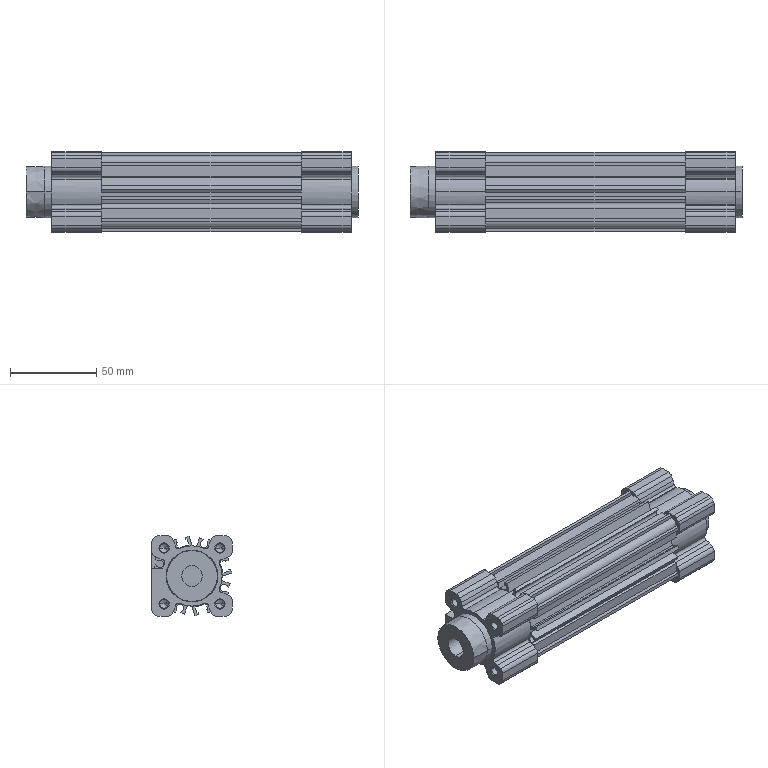Part | SolidWorks | features BaseBody 1 | 1 solid | 365 faces | box 193 x 47 x 47 mm | volume 214330 mm3 | plane 197 | cylinder 126 | cone 42 | commonest cylinder face diameters 6 x34 3 x18 4.917 x16 13.6 x14 4.25 x9 16.4 x8